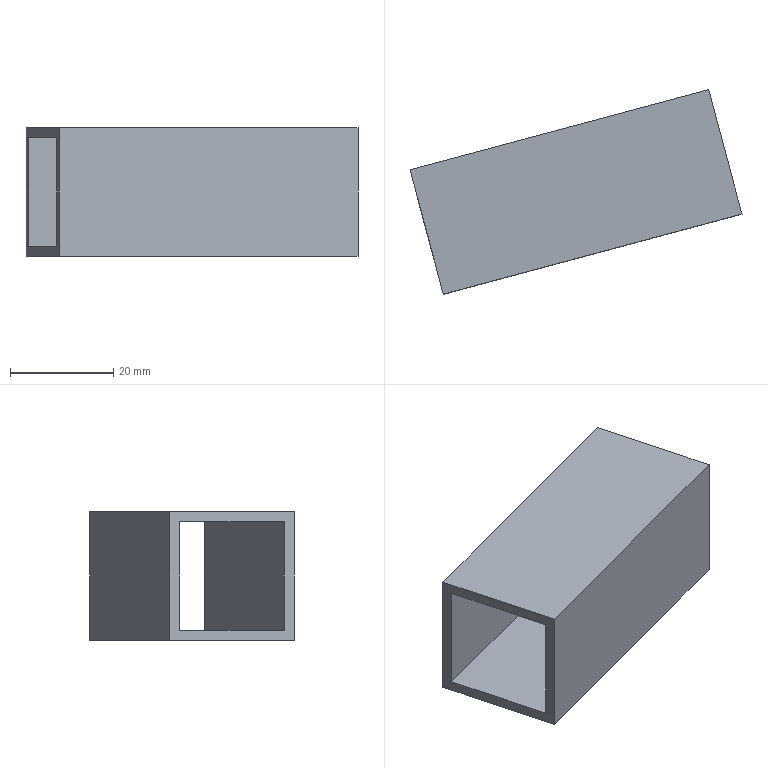Part | NX | features solid 2 | 1 solid | 10 faces | box 64.426 x 39.677 x 25 mm | volume 11040 mm3 | plane 10
STEP:
#1=CARTESIAN_POINT('',(-935.741,-113.852,20.));
#2=VERTEX_POINT('',#1);
#3=CARTESIAN_POINT('',(-935.741,-113.852,45.));
#4=VERTEX_POINT('',#3);
#5=CARTESIAN_POINT('',(-935.741,-113.852,20.));
#6=DIRECTION('',(0.,0.,1.));
#7=VECTOR('',#6,1000.);
#8=LINE('',#5,#7);
#9=EDGE_CURVE('',#2,#4,#8,.T.);
#10=ORIENTED_EDGE('',*,*,#9,.F.);
#11=CARTESIAN_POINT('',(-993.696,-129.382,20.));
#12=VERTEX_POINT('',#11);
#13=CARTESIAN_POINT('',(-839.148,-87.97,20.));
#14=DIRECTION('',(-0.9659,-0.2588,0.));
#15=VECTOR('',#14,1000.);
#16=LINE('',#13,#15);
#17=EDGE_CURVE('',#12,#2,#16,.F.);
#18=ORIENTED_EDGE('',*,*,#17,.F.);
#19=CARTESIAN_POINT('',(-993.696,-129.382,45.));
#20=VERTEX_POINT('',#19);
#21=CARTESIAN_POINT('',(-993.696,-129.382,20.));
#22=DIRECTION('',(0.,0.,1.));
#23=VECTOR('',#22,1000.);
#24=LINE('',#21,#23);
#25=EDGE_CURVE('',#12,#20,#24,.T.);
#26=ORIENTED_EDGE('',*,*,#25,.T.);
#27=CARTESIAN_POINT('',(-839.148,-87.97,45.));
#28=DIRECTION('',(-0.9659,-0.2588,0.));
#29=VECTOR('',#28,1000.);
#30=LINE('',#27,#29);
#31=EDGE_CURVE('',#20,#4,#30,.F.);
#32=ORIENTED_EDGE('',*,*,#31,.T.);
#33=EDGE_LOOP('',(#10,#18,#26,#32));
#34=FACE_BOUND('',#33,.T.);
#35=CARTESIAN_POINT('',(-839.148,-87.97,20.));
#36=DIRECTION('',(0.2588,-0.9659,0.));
#37=DIRECTION('',(0.,0.,1.));
#38=AXIS2_PLACEMENT_3D('',#35,#36,#37);
#39=PLANE('',#38);
#40=ADVANCED_FACE('',(#34),#39,.F.);
#41=CARTESIAN_POINT('',(-929.27,-138.001,45.));
#42=VERTEX_POINT('',#41);
#43=CARTESIAN_POINT('',(-935.741,-113.852,45.));
#44=DIRECTION('',(0.2588,-0.9659,0.));
#45=VECTOR('',#44,1000.);
#46=LINE('',#43,#45);
#47=EDGE_CURVE('',#4,#42,#46,.T.);
#48=ORIENTED_EDGE('',*,*,#47,.F.);
#49=ORIENTED_EDGE('',*,*,#31,.F.);
#50=CARTESIAN_POINT('',(-987.226,-153.53,45.));
#51=VERTEX_POINT('',#50);
#52=CARTESIAN_POINT('',(-993.696,-129.382,45.));
#53=DIRECTION('',(0.2588,-0.9659,0.));
#54=VECTOR('',#53,1000.);
#55=LINE('',#52,#54);
#56=EDGE_CURVE('',#20,#51,#55,.T.);
#57=ORIENTED_EDGE('',*,*,#56,.T.);
#58=CARTESIAN_POINT('',(-832.678,-112.119,45.));
#59=DIRECTION('',(-0.9659,-0.2588,0.));
#60=VECTOR('',#59,1000.);
#61=LINE('',#58,#60);
#62=EDGE_CURVE('',#51,#42,#61,.F.);
#63=ORIENTED_EDGE('',*,*,#62,.T.);
#64=EDGE_LOOP('',(#48,#49,#57,#63));
#65=FACE_BOUND('',#64,.T.);
#66=CARTESIAN_POINT('',(-839.148,-87.97,45.));
#67=DIRECTION('',(0.,0.,-1.));
#68=DIRECTION('',(0.2588,-0.9659,0.));
#69=AXIS2_PLACEMENT_3D('',#66,#67,#68);
#70=PLANE('',#69);
#71=ADVANCED_FACE('',(#65),#70,.F.);
#72=CARTESIAN_POINT('',(-929.27,-138.001,20.));
#73=VERTEX_POINT('',#72);
#74=CARTESIAN_POINT('',(-929.27,-138.001,20.));
#75=DIRECTION('',(0.,0.,1.));
#76=VECTOR('',#75,1000.);
#77=LINE('',#74,#76);
#78=EDGE_CURVE('',#42,#73,#77,.F.);
#79=ORIENTED_EDGE('',*,*,#78,.F.);
#80=ORIENTED_EDGE('',*,*,#62,.F.);
#81=CARTESIAN_POINT('',(-987.226,-153.53,20.));
#82=VERTEX_POINT('',#81);
#83=CARTESIAN_POINT('',(-987.226,-153.53,20.));
#84=DIRECTION('',(0.,0.,-1.));
#85=VECTOR('',#84,1000.);
#86=LINE('',#83,#85);
#87=EDGE_CURVE('',#82,#51,#86,.F.);
#88=ORIENTED_EDGE('',*,*,#87,.F.);
#89=CARTESIAN_POINT('',(-832.678,-112.119,20.));
#90=DIRECTION('',(-0.9659,-0.2588,0.));
#91=VECTOR('',#90,1000.);
#92=LINE('',#89,#91);
#93=EDGE_CURVE('',#82,#73,#92,.F.);
#94=ORIENTED_EDGE('',*,*,#93,.T.);
#95=EDGE_LOOP('',(#79,#80,#88,#94));
#96=FACE_BOUND('',#95,.T.);
#97=CARTESIAN_POINT('',(-832.678,-112.119,20.));
#98=DIRECTION('',(0.2588,-0.9659,0.));
#99=DIRECTION('',(0.,0.,1.));
#100=AXIS2_PLACEMENT_3D('',#97,#98,#99);
#101=PLANE('',#100);
#102=ADVANCED_FACE('',(#96),#101,.T.);
#103=CARTESIAN_POINT('',(-935.741,-113.852,20.));
#104=DIRECTION('',(0.2588,-0.9659,0.));
#105=VECTOR('',#104,1000.);
#106=LINE('',#103,#105);
#107=EDGE_CURVE('',#73,#2,#106,.F.);
#108=ORIENTED_EDGE('',*,*,#107,.F.);
#109=ORIENTED_EDGE('',*,*,#93,.F.);
#110=CARTESIAN_POINT('',(-993.696,-129.382,20.));
#111=DIRECTION('',(-0.2588,0.9659,0.));
#112=VECTOR('',#111,1000.);
#113=LINE('',#110,#112);
#114=EDGE_CURVE('',#12,#82,#113,.F.);
#115=ORIENTED_EDGE('',*,*,#114,.F.);
#116=ORIENTED_EDGE('',*,*,#17,.T.);
#117=EDGE_LOOP('',(#108,#109,#115,#116));
#118=FACE_BOUND('',#117,.T.);
#119=CARTESIAN_POINT('',(-839.148,-87.97,20.));
#120=DIRECTION('',(0.,0.,-1.));
#121=DIRECTION('',(0.2588,-0.9659,0.));
#122=AXIS2_PLACEMENT_3D('',#119,#120,#121);
#123=PLANE('',#122);
#124=ADVANCED_FACE('',(#118),#123,.T.);
#125=ORIENTED_EDGE('',*,*,#56,.F.);
#126=ORIENTED_EDGE('',*,*,#25,.F.);
#127=ORIENTED_EDGE('',*,*,#114,.T.);
#128=ORIENTED_EDGE('',*,*,#87,.T.);
#129=EDGE_LOOP('',(#125,#126,#127,#128));
#130=FACE_BOUND('',#129,.T.);
#131=CARTESIAN_POINT('',(-993.179,-131.313,22.));
#132=VERTEX_POINT('',#131);
#133=CARTESIAN_POINT('',(-993.179,-131.313,43.));
#134=VERTEX_POINT('',#133);
#135=CARTESIAN_POINT('',(-993.179,-131.313,20.));
#136=DIRECTION('',(0.,0.,1.));
#137=VECTOR('',#136,1000.);
#138=LINE('',#135,#137);
#139=EDGE_CURVE('',#132,#134,#138,.T.);
#140=ORIENTED_EDGE('',*,*,#139,.T.);
#141=CARTESIAN_POINT('',(-987.743,-151.598,43.));
#142=VERTEX_POINT('',#141);
#143=CARTESIAN_POINT('',(-993.696,-129.382,43.));
#144=DIRECTION('',(0.2588,-0.9659,0.));
#145=VECTOR('',#144,1000.);
#146=LINE('',#143,#145);
#147=EDGE_CURVE('',#134,#142,#146,.T.);
#148=ORIENTED_EDGE('',*,*,#147,.T.);
#149=CARTESIAN_POINT('',(-987.743,-151.598,22.));
#150=VERTEX_POINT('',#149);
#151=CARTESIAN_POINT('',(-987.743,-151.598,20.));
#152=DIRECTION('',(0.,0.,-1.));
#153=VECTOR('',#152,1000.);
#154=LINE('',#151,#153);
#155=EDGE_CURVE('',#150,#142,#154,.F.);
#156=ORIENTED_EDGE('',*,*,#155,.F.);
#157=CARTESIAN_POINT('',(-993.696,-129.382,22.));
#158=DIRECTION('',(-0.2588,0.9659,0.));
#159=VECTOR('',#158,1000.);
#160=LINE('',#157,#159);
#161=EDGE_CURVE('',#132,#150,#160,.F.);
#162=ORIENTED_EDGE('',*,*,#161,.F.);
#163=EDGE_LOOP('',(#140,#148,#156,#162));
#164=FACE_BOUND('',#163,.T.);
#165=CARTESIAN_POINT('',(-993.696,-129.382,20.));
#166=DIRECTION('',(-0.9659,-0.2588,0.));
#167=DIRECTION('',(0.,0.,1.));
#168=AXIS2_PLACEMENT_3D('',#165,#166,#167);
#169=PLANE('',#168);
#170=ADVANCED_FACE('',(#130,#164),#169,.T.);
#171=CARTESIAN_POINT('',(-935.223,-115.784,22.));
#172=VERTEX_POINT('',#171);
#173=CARTESIAN_POINT('',(-838.631,-89.902,22.));
#174=DIRECTION('',(-0.9659,-0.2588,0.));
#175=VECTOR('',#174,1000.);
#176=LINE('',#173,#175);
#177=EDGE_CURVE('',#132,#172,#176,.F.);
#178=ORIENTED_EDGE('',*,*,#177,.T.);
#179=CARTESIAN_POINT('',(-935.223,-115.784,43.));
#180=VERTEX_POINT('',#179);
#181=CARTESIAN_POINT('',(-935.223,-115.784,20.));
#182=DIRECTION('',(0.,0.,1.));
#183=VECTOR('',#182,1000.);
#184=LINE('',#181,#183);
#185=EDGE_CURVE('',#172,#180,#184,.T.);
#186=ORIENTED_EDGE('',*,*,#185,.T.);
#187=CARTESIAN_POINT('',(-838.631,-89.902,43.));
#188=DIRECTION('',(0.9659,0.2588,0.));
#189=VECTOR('',#188,1000.);
#190=LINE('',#187,#189);
#191=EDGE_CURVE('',#134,#180,#190,.T.);
#192=ORIENTED_EDGE('',*,*,#191,.F.);
#193=ORIENTED_EDGE('',*,*,#139,.F.);
#194=EDGE_LOOP('',(#178,#186,#192,#193));
#195=FACE_BOUND('',#194,.T.);
#196=CARTESIAN_POINT('',(-838.631,-89.902,20.));
#197=DIRECTION('',(0.2588,-0.9659,0.));
#198=DIRECTION('',(0.,0.,1.));
#199=AXIS2_PLACEMENT_3D('',#196,#197,#198);
#200=PLANE('',#199);
#201=ADVANCED_FACE('',(#195),#200,.T.);
#202=ORIENTED_EDGE('',*,*,#191,.T.);
#203=CARTESIAN_POINT('',(-929.788,-136.069,43.));
#204=VERTEX_POINT('',#203);
#205=CARTESIAN_POINT('',(-935.741,-113.852,43.));
#206=DIRECTION('',(0.2588,-0.9659,0.));
#207=VECTOR('',#206,1000.);
#208=LINE('',#205,#207);
#209=EDGE_CURVE('',#180,#204,#208,.T.);
#210=ORIENTED_EDGE('',*,*,#209,.T.);
#211=CARTESIAN_POINT('',(-833.195,-110.187,43.));
#212=DIRECTION('',(-0.9659,-0.2588,0.));
#213=VECTOR('',#212,1000.);
#214=LINE('',#211,#213);
#215=EDGE_CURVE('',#142,#204,#214,.F.);
#216=ORIENTED_EDGE('',*,*,#215,.F.);
#217=ORIENTED_EDGE('',*,*,#147,.F.);
#218=EDGE_LOOP('',(#202,#210,#216,#217));
#219=FACE_BOUND('',#218,.T.);
#220=CARTESIAN_POINT('',(-839.148,-87.97,43.));
#221=DIRECTION('',(0.,0.,-1.));
#222=DIRECTION('',(0.2588,-0.9659,0.));
#223=AXIS2_PLACEMENT_3D('',#220,#221,#222);
#224=PLANE('',#223);
#225=ADVANCED_FACE('',(#219),#224,.T.);
#226=ORIENTED_EDGE('',*,*,#215,.T.);
#227=CARTESIAN_POINT('',(-929.788,-136.069,22.));
#228=VERTEX_POINT('',#227);
#229=CARTESIAN_POINT('',(-929.788,-136.069,20.));
#230=DIRECTION('',(0.,0.,1.));
#231=VECTOR('',#230,1000.);
#232=LINE('',#229,#231);
#233=EDGE_CURVE('',#204,#228,#232,.F.);
#234=ORIENTED_EDGE('',*,*,#233,.T.);
#235=CARTESIAN_POINT('',(-833.195,-110.187,22.));
#236=DIRECTION('',(0.9659,0.2588,0.));
#237=VECTOR('',#236,1000.);
#238=LINE('',#235,#237);
#239=EDGE_CURVE('',#150,#228,#238,.T.);
#240=ORIENTED_EDGE('',*,*,#239,.F.);
#241=ORIENTED_EDGE('',*,*,#155,.T.);
#242=EDGE_LOOP('',(#226,#234,#240,#241));
#243=FACE_BOUND('',#242,.T.);
#244=CARTESIAN_POINT('',(-833.195,-110.187,20.));
#245=DIRECTION('',(0.2588,-0.9659,0.));
#246=DIRECTION('',(0.,0.,1.));
#247=AXIS2_PLACEMENT_3D('',#244,#245,#246);
#248=PLANE('',#247);
#249=ADVANCED_FACE('',(#243),#248,.F.);
#250=ORIENTED_EDGE('',*,*,#239,.T.);
#251=CARTESIAN_POINT('',(-935.741,-113.852,22.));
#252=DIRECTION('',(0.2588,-0.9659,0.));
#253=VECTOR('',#252,1000.);
#254=LINE('',#251,#253);
#255=EDGE_CURVE('',#228,#172,#254,.F.);
#256=ORIENTED_EDGE('',*,*,#255,.T.);
#257=ORIENTED_EDGE('',*,*,#177,.F.);
#258=ORIENTED_EDGE('',*,*,#161,.T.);
#259=EDGE_LOOP('',(#250,#256,#257,#258));
#260=FACE_BOUND('',#259,.T.);
#261=CARTESIAN_POINT('',(-839.148,-87.97,22.));
#262=DIRECTION('',(0.,0.,-1.));
#263=DIRECTION('',(0.2588,-0.9659,0.));
#264=AXIS2_PLACEMENT_3D('',#261,#262,#263);
#265=PLANE('',#264);
#266=ADVANCED_FACE('',(#260),#265,.F.);
#267=ORIENTED_EDGE('',*,*,#255,.F.);
#268=ORIENTED_EDGE('',*,*,#233,.F.);
#269=ORIENTED_EDGE('',*,*,#209,.F.);
#270=ORIENTED_EDGE('',*,*,#185,.F.);
#271=EDGE_LOOP('',(#267,#268,#269,#270));
#272=FACE_BOUND('',#271,.T.);
#273=ORIENTED_EDGE('',*,*,#78,.T.);
#274=ORIENTED_EDGE('',*,*,#107,.T.);
#275=ORIENTED_EDGE('',*,*,#9,.T.);
#276=ORIENTED_EDGE('',*,*,#47,.T.);
#277=EDGE_LOOP('',(#273,#274,#275,#276));
#278=FACE_BOUND('',#277,.T.);
#279=CARTESIAN_POINT('',(-935.741,-113.852,90.969));
#280=DIRECTION('',(0.9659,0.2588,0.));
#281=DIRECTION('',(-0.2588,0.9659,0.));
#282=AXIS2_PLACEMENT_3D('',#279,#280,#281);
#283=PLANE('',#282);
#284=ADVANCED_FACE('',(#272,#278),#283,.T.);
#285=CLOSED_SHELL('',(#40,#71,#102,#124,#170,#201,#225,#249,#266,#284));
#286=MANIFOLD_SOLID_BREP('',#285);
#287=(LENGTH_UNIT()NAMED_UNIT(*)SI_UNIT(.MILLI.,.METRE.));
#288=UNCERTAINTY_MEASURE_WITH_UNIT(LENGTH_MEASURE(0.00001),#287,'','');
#289=(NAMED_UNIT(*)PLANE_ANGLE_UNIT()SI_UNIT($,.RADIAN.));
#290=(NAMED_UNIT(*)SI_UNIT($,.STERADIAN.)SOLID_ANGLE_UNIT());
#291=(GEOMETRIC_REPRESENTATION_CONTEXT(3)GLOBAL_UNCERTAINTY_ASSIGNED_CONTEXT((#288))GLOBAL_UNIT_ASSIGNED_CONTEXT((#287,#289,#290))REPRESENTATION_CONTEXT('',''));
#292=ADVANCED_BREP_SHAPE_REPRESENTATION('',(#286),#291);